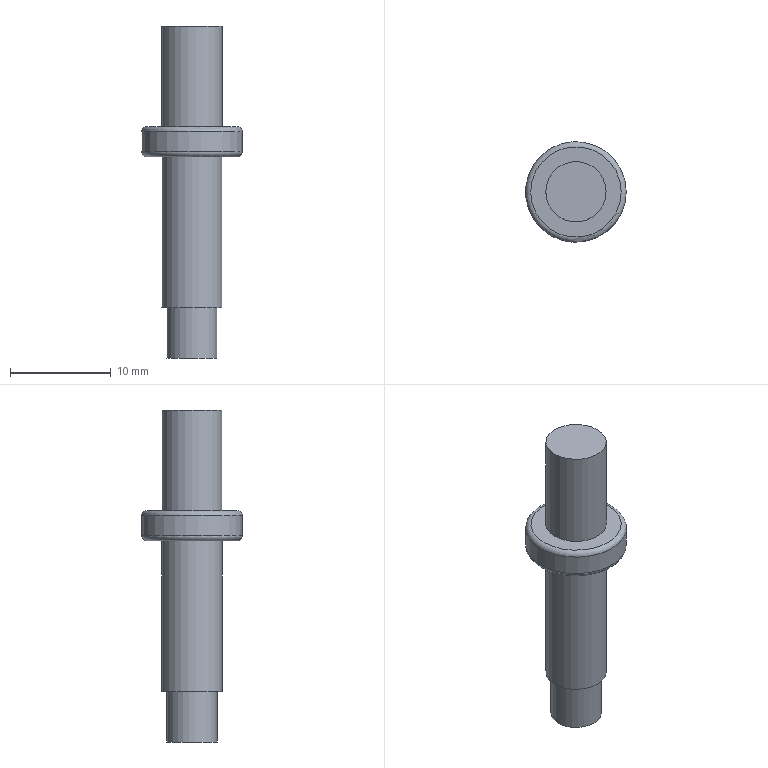Part | STEP file | 1-01.14 | 1 solid | 11 faces | box 10 x 10 x 33 mm | volume 1037 mm3 | plane 5 | cylinder 4 | torus 2 | commonest cylinder face diameters 6 x2 5 x1 10 x1
STEP:
#1=CARTESIAN_POINT('',(0.,0.,0.));
#2=DIRECTION('',(0.,0.,1.));
#3=DIRECTION('',(1.,0.,0.));
#4=AXIS2_PLACEMENT_3D('',#1,#2,#3);
#5=CARTESIAN_POINT('',(3.,0.,10.));
#6=VERTEX_POINT('',#5);
#7=CARTESIAN_POINT('',(0.,0.,10.));
#8=DIRECTION('',(0.,0.,1.));
#9=DIRECTION('',(1.,0.,0.));
#10=AXIS2_PLACEMENT_3D('',#7,#8,#9);
#11=CIRCLE('',#10,3.);
#12=CARTESIAN_POINT('',(-0.8038,0.,10.));
#13=DIRECTION('',(0.,0.,1.));
#14=DIRECTION('',(1.,0.,0.));
#15=AXIS2_PLACEMENT_3D('',#12,#13,#14);
#16=PLANE('',#15);
#17=CARTESIAN_POINT('',(0.8038,0.));
#18=DIRECTION('',(1.,0.));
#19=AXIS2_PLACEMENT_2D('',#17,#18);
#20=CIRCLE('',#19,3.);
#21=(GEOMETRIC_REPRESENTATION_CONTEXT(2)PARAMETRIC_REPRESENTATION_CONTEXT()REPRESENTATION_CONTEXT('',''));
#22=DEFINITIONAL_REPRESENTATION('',(#20),#21);
#23=PCURVE('',#16,#22);
#24=CARTESIAN_POINT('',(0.,0.,0.));
#25=DIRECTION('',(0.,0.,1.));
#26=DIRECTION('',(1.,0.,0.));
#27=AXIS2_PLACEMENT_3D('',#24,#25,#26);
#28=CYLINDRICAL_SURFACE('',#27,3.);
#29=CARTESIAN_POINT('',(0.,10.));
#30=DIRECTION('',(1.,0.));
#31=VECTOR('',#30,1.);
#32=LINE('',#29,#31);
#33=(GEOMETRIC_REPRESENTATION_CONTEXT(2)PARAMETRIC_REPRESENTATION_CONTEXT()REPRESENTATION_CONTEXT('',''));
#34=DEFINITIONAL_REPRESENTATION('',(#32),#33);
#35=PCURVE('',#28,#34);
#36=SURFACE_CURVE('',#11,(#23,#35),.PCURVE_S1.);
#37=EDGE_CURVE('',#6,#6,#36,.T.);
#38=ORIENTED_EDGE('',*,*,#37,.T.);
#39=EDGE_LOOP('',(#38));
#40=FACE_BOUND('',#39,.T.);
#41=ADVANCED_FACE('',(#40),#16,.T.);
#42=CARTESIAN_POINT('',(3.,0.,0.));
#43=VERTEX_POINT('',#42);
#44=CARTESIAN_POINT('',(0.,0.,0.));
#45=DIRECTION('',(0.,0.,1.));
#46=DIRECTION('',(1.,0.,0.));
#47=AXIS2_PLACEMENT_3D('',#44,#45,#46);
#48=CIRCLE('',#47,3.);
#49=CARTESIAN_POINT('',(0.,0.));
#50=DIRECTION('',(1.,0.));
#51=VECTOR('',#50,1.);
#52=LINE('',#49,#51);
#53=(GEOMETRIC_REPRESENTATION_CONTEXT(2)PARAMETRIC_REPRESENTATION_CONTEXT()REPRESENTATION_CONTEXT('',''));
#54=DEFINITIONAL_REPRESENTATION('',(#52),#53);
#55=PCURVE('',#28,#54);
#56=CARTESIAN_POINT('',(-1.34,0.,0.));
#57=DIRECTION('',(0.,0.,1.));
#58=DIRECTION('',(1.,0.,0.));
#59=AXIS2_PLACEMENT_3D('',#56,#57,#58);
#60=PLANE('',#59);
#61=CARTESIAN_POINT('',(1.34,0.));
#62=DIRECTION('',(1.,0.));
#63=AXIS2_PLACEMENT_2D('',#61,#62);
#64=CIRCLE('',#63,3.);
#65=(GEOMETRIC_REPRESENTATION_CONTEXT(2)PARAMETRIC_REPRESENTATION_CONTEXT()REPRESENTATION_CONTEXT('',''));
#66=DEFINITIONAL_REPRESENTATION('',(#64),#65);
#67=PCURVE('',#60,#66);
#68=SURFACE_CURVE('',#48,(#55,#67),.PCURVE_S1.);
#69=EDGE_CURVE('',#43,#43,#68,.T.);
#70=ORIENTED_EDGE('',*,*,#69,.T.);
#71=CARTESIAN_POINT('',(3.,0.,0.));
#72=DIRECTION('',(0.,0.,1.));
#73=VECTOR('',#72,1.);
#74=LINE('',#71,#73);
#75=CARTESIAN_POINT('',(6.283,0.));
#76=DIRECTION('',(0.,1.));
#77=VECTOR('',#76,1.);
#78=LINE('',#75,#77);
#79=(GEOMETRIC_REPRESENTATION_CONTEXT(2)PARAMETRIC_REPRESENTATION_CONTEXT()REPRESENTATION_CONTEXT('',''));
#80=DEFINITIONAL_REPRESENTATION('',(#78),#79);
#81=PCURVE('',#28,#80);
#82=CARTESIAN_POINT('',(0.,0.));
#83=DIRECTION('',(0.,1.));
#84=VECTOR('',#83,1.);
#85=LINE('',#82,#84);
#86=(GEOMETRIC_REPRESENTATION_CONTEXT(2)PARAMETRIC_REPRESENTATION_CONTEXT()REPRESENTATION_CONTEXT('',''));
#87=DEFINITIONAL_REPRESENTATION('',(#85),#86);
#88=PCURVE('',#28,#87);
#89=SEAM_CURVE('',#74,(#81,#88),.PCURVE_S1.);
#90=EDGE_CURVE('',#43,#6,#89,.T.);
#91=ORIENTED_EDGE('',*,*,#90,.T.);
#92=ORIENTED_EDGE('',*,*,#37,.F.);
#93=ORIENTED_EDGE('',*,*,#90,.F.);
#94=EDGE_LOOP('',(#70,#91,#92,#93));
#95=FACE_BOUND('',#94,.T.);
#96=ADVANCED_FACE('',(#95),#28,.T.);
#97=CARTESIAN_POINT('',(0.,-3.,-3.));
#98=VERTEX_POINT('',#97);
#99=CARTESIAN_POINT('',(0.,0.,-3.));
#100=DIRECTION('',(0.,0.,-1.));
#101=DIRECTION('',(0.,-1.,0.));
#102=AXIS2_PLACEMENT_3D('',#99,#100,#101);
#103=CIRCLE('',#102,3.);
#104=CARTESIAN_POINT('',(0.,0.,-3.));
#105=DIRECTION('',(0.,0.,-1.));
#106=DIRECTION('',(0.,-1.,0.));
#107=AXIS2_PLACEMENT_3D('',#104,#105,#106);
#108=CYLINDRICAL_SURFACE('',#107,3.);
#109=CARTESIAN_POINT('',(0.,0.));
#110=DIRECTION('',(1.,0.));
#111=VECTOR('',#110,1.);
#112=LINE('',#109,#111);
#113=(GEOMETRIC_REPRESENTATION_CONTEXT(2)PARAMETRIC_REPRESENTATION_CONTEXT()REPRESENTATION_CONTEXT('',''));
#114=DEFINITIONAL_REPRESENTATION('',(#112),#113);
#115=PCURVE('',#108,#114);
#116=CARTESIAN_POINT('',(-1.34,0.,-3.));
#117=DIRECTION('',(0.,0.,1.));
#118=DIRECTION('',(1.,0.,0.));
#119=AXIS2_PLACEMENT_3D('',#116,#117,#118);
#120=PLANE('',#119);
#121=CARTESIAN_POINT('',(1.34,-3.));
#122=CARTESIAN_POINT('',(-3.856,-3.));
#123=CARTESIAN_POINT('',(-1.258,1.5));
#124=CARTESIAN_POINT('',(1.34,6.));
#125=CARTESIAN_POINT('',(3.938,1.5));
#126=CARTESIAN_POINT('',(6.536,-3.));
#127=CARTESIAN_POINT('',(1.34,-3.));
#128=(BOUNDED_CURVE()B_SPLINE_CURVE(2,(#121,#122,#123,#124,#125,#126,#127),.UNSPECIFIED.,.T.,.F.)B_SPLINE_CURVE_WITH_KNOTS((1,2,2,2,2,1),(-2.094,0.,2.094,4.189,6.283,8.378),.UNSPECIFIED.)CURVE()GEOMETRIC_REPRESENTATION_ITEM()RATIONAL_B_SPLINE_CURVE((1.,0.5,1.,0.5,1.,0.5,1.))REPRESENTATION_ITEM(''));
#129=(GEOMETRIC_REPRESENTATION_CONTEXT(2)PARAMETRIC_REPRESENTATION_CONTEXT()REPRESENTATION_CONTEXT('',''));
#130=DEFINITIONAL_REPRESENTATION('',(#128),#129);
#131=PCURVE('',#120,#130);
#132=SURFACE_CURVE('',#103,(#115,#131),.PCURVE_S1.);
#133=EDGE_CURVE('',#98,#98,#132,.T.);
#134=ORIENTED_EDGE('',*,*,#133,.T.);
#135=CARTESIAN_POINT('',(0.,-3.,-18.));
#136=VERTEX_POINT('',#135);
#137=CARTESIAN_POINT('',(0.,-3.,-3.));
#138=DIRECTION('',(0.,0.,-1.));
#139=VECTOR('',#138,1.);
#140=LINE('',#137,#139);
#141=CARTESIAN_POINT('',(6.283,0.));
#142=DIRECTION('',(0.,1.));
#143=VECTOR('',#142,1.);
#144=LINE('',#141,#143);
#145=(GEOMETRIC_REPRESENTATION_CONTEXT(2)PARAMETRIC_REPRESENTATION_CONTEXT()REPRESENTATION_CONTEXT('',''));
#146=DEFINITIONAL_REPRESENTATION('',(#144),#145);
#147=PCURVE('',#108,#146);
#148=CARTESIAN_POINT('',(0.,0.));
#149=DIRECTION('',(0.,1.));
#150=VECTOR('',#149,1.);
#151=LINE('',#148,#150);
#152=(GEOMETRIC_REPRESENTATION_CONTEXT(2)PARAMETRIC_REPRESENTATION_CONTEXT()REPRESENTATION_CONTEXT('',''));
#153=DEFINITIONAL_REPRESENTATION('',(#151),#152);
#154=PCURVE('',#108,#153);
#155=SEAM_CURVE('',#140,(#147,#154),.PCURVE_S1.);
#156=EDGE_CURVE('',#98,#136,#155,.T.);
#157=ORIENTED_EDGE('',*,*,#156,.T.);
#158=CARTESIAN_POINT('',(0.,0.,-18.));
#159=DIRECTION('',(0.,0.,-1.));
#160=DIRECTION('',(0.,-1.,0.));
#161=AXIS2_PLACEMENT_3D('',#158,#159,#160);
#162=CIRCLE('',#161,3.);
#163=CARTESIAN_POINT('',(0.,15.));
#164=DIRECTION('',(1.,0.));
#165=VECTOR('',#164,1.);
#166=LINE('',#163,#165);
#167=(GEOMETRIC_REPRESENTATION_CONTEXT(2)PARAMETRIC_REPRESENTATION_CONTEXT()REPRESENTATION_CONTEXT('',''));
#168=DEFINITIONAL_REPRESENTATION('',(#166),#167);
#169=PCURVE('',#108,#168);
#170=CARTESIAN_POINT('',(0.,0.8038,-18.));
#171=DIRECTION('',(0.,0.,-1.));
#172=DIRECTION('',(0.,-1.,0.));
#173=AXIS2_PLACEMENT_3D('',#170,#171,#172);
#174=PLANE('',#173);
#175=CARTESIAN_POINT('',(0.8038,0.));
#176=DIRECTION('',(1.,0.));
#177=AXIS2_PLACEMENT_2D('',#175,#176);
#178=CIRCLE('',#177,3.);
#179=(GEOMETRIC_REPRESENTATION_CONTEXT(2)PARAMETRIC_REPRESENTATION_CONTEXT()REPRESENTATION_CONTEXT('',''));
#180=DEFINITIONAL_REPRESENTATION('',(#178),#179);
#181=PCURVE('',#174,#180);
#182=SURFACE_CURVE('',#162,(#169,#181),.PCURVE_S1.);
#183=EDGE_CURVE('',#136,#136,#182,.T.);
#184=ORIENTED_EDGE('',*,*,#183,.F.);
#185=ORIENTED_EDGE('',*,*,#156,.F.);
#186=EDGE_LOOP('',(#134,#157,#184,#185));
#187=FACE_BOUND('',#186,.T.);
#188=ADVANCED_FACE('',(#187),#108,.T.);
#189=ORIENTED_EDGE('',*,*,#183,.T.);
#190=EDGE_LOOP('',(#189));
#191=FACE_BOUND('',#190,.T.);
#192=CARTESIAN_POINT('',(0.,-2.5,-18.));
#193=VERTEX_POINT('',#192);
#194=CARTESIAN_POINT('',(0.,0.,-18.));
#195=DIRECTION('',(0.,0.,-1.));
#196=DIRECTION('',(0.,-1.,0.));
#197=AXIS2_PLACEMENT_3D('',#194,#195,#196);
#198=CIRCLE('',#197,2.5);
#199=CARTESIAN_POINT('',(0.8038,0.));
#200=DIRECTION('',(1.,0.));
#201=AXIS2_PLACEMENT_2D('',#199,#200);
#202=CIRCLE('',#201,2.5);
#203=(GEOMETRIC_REPRESENTATION_CONTEXT(2)PARAMETRIC_REPRESENTATION_CONTEXT()REPRESENTATION_CONTEXT('',''));
#204=DEFINITIONAL_REPRESENTATION('',(#202),#203);
#205=PCURVE('',#174,#204);
#206=CARTESIAN_POINT('',(0.,0.,-18.));
#207=DIRECTION('',(0.,0.,-1.));
#208=DIRECTION('',(0.,-1.,0.));
#209=AXIS2_PLACEMENT_3D('',#206,#207,#208);
#210=CYLINDRICAL_SURFACE('',#209,2.5);
#211=CARTESIAN_POINT('',(0.,0.));
#212=DIRECTION('',(1.,0.));
#213=VECTOR('',#212,1.);
#214=LINE('',#211,#213);
#215=(GEOMETRIC_REPRESENTATION_CONTEXT(2)PARAMETRIC_REPRESENTATION_CONTEXT()REPRESENTATION_CONTEXT('',''));
#216=DEFINITIONAL_REPRESENTATION('',(#214),#215);
#217=PCURVE('',#210,#216);
#218=SURFACE_CURVE('',#198,(#205,#217),.PCURVE_S1.);
#219=EDGE_CURVE('',#193,#193,#218,.T.);
#220=ORIENTED_EDGE('',*,*,#219,.F.);
#221=EDGE_LOOP('',(#220));
#222=FACE_BOUND('',#221,.T.);
#223=ADVANCED_FACE('',(#191,#222),#174,.T.);
#224=ORIENTED_EDGE('',*,*,#219,.T.);
#225=CARTESIAN_POINT('',(0.,-2.5,-23.));
#226=VERTEX_POINT('',#225);
#227=CARTESIAN_POINT('',(0.,-2.5,-18.));
#228=DIRECTION('',(0.,0.,-1.));
#229=VECTOR('',#228,1.);
#230=LINE('',#227,#229);
#231=CARTESIAN_POINT('',(6.283,0.));
#232=DIRECTION('',(0.,1.));
#233=VECTOR('',#232,1.);
#234=LINE('',#231,#233);
#235=(GEOMETRIC_REPRESENTATION_CONTEXT(2)PARAMETRIC_REPRESENTATION_CONTEXT()REPRESENTATION_CONTEXT('',''));
#236=DEFINITIONAL_REPRESENTATION('',(#234),#235);
#237=PCURVE('',#210,#236);
#238=CARTESIAN_POINT('',(0.,0.));
#239=DIRECTION('',(0.,1.));
#240=VECTOR('',#239,1.);
#241=LINE('',#238,#240);
#242=(GEOMETRIC_REPRESENTATION_CONTEXT(2)PARAMETRIC_REPRESENTATION_CONTEXT()REPRESENTATION_CONTEXT('',''));
#243=DEFINITIONAL_REPRESENTATION('',(#241),#242);
#244=PCURVE('',#210,#243);
#245=SEAM_CURVE('',#230,(#237,#244),.PCURVE_S1.);
#246=EDGE_CURVE('',#193,#226,#245,.T.);
#247=ORIENTED_EDGE('',*,*,#246,.T.);
#248=CARTESIAN_POINT('',(0.,0.,-23.));
#249=DIRECTION('',(0.,0.,-1.));
#250=DIRECTION('',(0.,-1.,0.));
#251=AXIS2_PLACEMENT_3D('',#248,#249,#250);
#252=CIRCLE('',#251,2.5);
#253=CARTESIAN_POINT('',(0.,5.));
#254=DIRECTION('',(1.,0.));
#255=VECTOR('',#254,1.);
#256=LINE('',#253,#255);
#257=(GEOMETRIC_REPRESENTATION_CONTEXT(2)PARAMETRIC_REPRESENTATION_CONTEXT()REPRESENTATION_CONTEXT('',''));
#258=DEFINITIONAL_REPRESENTATION('',(#256),#257);
#259=PCURVE('',#210,#258);
#260=CARTESIAN_POINT('',(0.,0.6699,-23.));
#261=DIRECTION('',(0.,0.,-1.));
#262=DIRECTION('',(0.,-1.,0.));
#263=AXIS2_PLACEMENT_3D('',#260,#261,#262);
#264=PLANE('',#263);
#265=CARTESIAN_POINT('',(0.6699,0.));
#266=DIRECTION('',(1.,0.));
#267=AXIS2_PLACEMENT_2D('',#265,#266);
#268=CIRCLE('',#267,2.5);
#269=(GEOMETRIC_REPRESENTATION_CONTEXT(2)PARAMETRIC_REPRESENTATION_CONTEXT()REPRESENTATION_CONTEXT('',''));
#270=DEFINITIONAL_REPRESENTATION('',(#268),#269);
#271=PCURVE('',#264,#270);
#272=SURFACE_CURVE('',#252,(#259,#271),.PCURVE_S1.);
#273=EDGE_CURVE('',#226,#226,#272,.T.);
#274=ORIENTED_EDGE('',*,*,#273,.F.);
#275=ORIENTED_EDGE('',*,*,#246,.F.);
#276=EDGE_LOOP('',(#224,#247,#274,#275));
#277=FACE_BOUND('',#276,.T.);
#278=ADVANCED_FACE('',(#277),#210,.T.);
#279=ORIENTED_EDGE('',*,*,#273,.T.);
#280=EDGE_LOOP('',(#279));
#281=FACE_BOUND('',#280,.T.);
#282=ADVANCED_FACE('',(#281),#264,.T.);
#283=CARTESIAN_POINT('',(4.5,0.,0.));
#284=VERTEX_POINT('',#283);
#285=CARTESIAN_POINT('',(0.,0.,0.));
#286=DIRECTION('',(0.,0.,1.));
#287=DIRECTION('',(1.,0.,0.));
#288=AXIS2_PLACEMENT_3D('',#285,#286,#287);
#289=CIRCLE('',#288,4.5);
#290=CARTESIAN_POINT('',(1.34,0.));
#291=DIRECTION('',(1.,0.));
#292=AXIS2_PLACEMENT_2D('',#290,#291);
#293=CIRCLE('',#292,4.5);
#294=(GEOMETRIC_REPRESENTATION_CONTEXT(2)PARAMETRIC_REPRESENTATION_CONTEXT()REPRESENTATION_CONTEXT('',''));
#295=DEFINITIONAL_REPRESENTATION('',(#293),#294);
#296=PCURVE('',#60,#295);
#297=CARTESIAN_POINT('',(0.,0.,-0.5));
#298=DIRECTION('',(0.,0.,-1.));
#299=DIRECTION('',(1.,0.,0.));
#300=AXIS2_PLACEMENT_3D('',#297,#298,#299);
#301=TOROIDAL_SURFACE('',#300,4.5,0.5);
#302=CARTESIAN_POINT('',(6.283,4.712));
#303=DIRECTION('',(-1.,0.));
#304=VECTOR('',#303,1.);
#305=LINE('',#302,#304);
#306=(GEOMETRIC_REPRESENTATION_CONTEXT(2)PARAMETRIC_REPRESENTATION_CONTEXT()REPRESENTATION_CONTEXT('',''));
#307=DEFINITIONAL_REPRESENTATION('',(#305),#306);
#308=PCURVE('',#301,#307);
#309=SURFACE_CURVE('',#289,(#296,#308),.PCURVE_S1.);
#310=EDGE_CURVE('',#284,#284,#309,.T.);
#311=ORIENTED_EDGE('',*,*,#310,.T.);
#312=EDGE_LOOP('',(#311));
#313=FACE_BOUND('',#312,.T.);
#314=ORIENTED_EDGE('',*,*,#69,.F.);
#315=EDGE_LOOP('',(#314));
#316=FACE_BOUND('',#315,.T.);
#317=ADVANCED_FACE('',(#313,#316),#60,.T.);
#318=CARTESIAN_POINT('',(5.,0.,-0.5));
#319=VERTEX_POINT('',#318);
#320=CARTESIAN_POINT('',(0.,0.,-0.5));
#321=DIRECTION('',(0.,0.,1.));
#322=DIRECTION('',(1.,0.,0.));
#323=AXIS2_PLACEMENT_3D('',#320,#321,#322);
#324=CIRCLE('',#323,5.);
#325=CARTESIAN_POINT('',(0.,0.,0.));
#326=DIRECTION('',(0.,0.,-1.));
#327=DIRECTION('',(1.,0.,0.));
#328=AXIS2_PLACEMENT_3D('',#325,#326,#327);
#329=CYLINDRICAL_SURFACE('',#328,5.);
#330=CARTESIAN_POINT('',(6.283,0.5));
#331=DIRECTION('',(-1.,0.));
#332=VECTOR('',#331,1.);
#333=LINE('',#330,#332);
#334=(GEOMETRIC_REPRESENTATION_CONTEXT(2)PARAMETRIC_REPRESENTATION_CONTEXT()REPRESENTATION_CONTEXT('',''));
#335=DEFINITIONAL_REPRESENTATION('',(#333),#334);
#336=PCURVE('',#329,#335);
#337=CARTESIAN_POINT('',(6.283,6.283));
#338=DIRECTION('',(-1.,0.));
#339=VECTOR('',#338,1.);
#340=LINE('',#337,#339);
#341=(GEOMETRIC_REPRESENTATION_CONTEXT(2)PARAMETRIC_REPRESENTATION_CONTEXT()REPRESENTATION_CONTEXT('',''));
#342=DEFINITIONAL_REPRESENTATION('',(#340),#341);
#343=PCURVE('',#301,#342);
#344=SURFACE_CURVE('',#324,(#336,#343),.PCURVE_S1.);
#345=EDGE_CURVE('',#319,#319,#344,.T.);
#346=ORIENTED_EDGE('',*,*,#345,.F.);
#347=CARTESIAN_POINT('',(5.,0.,-2.5));
#348=VERTEX_POINT('',#347);
#349=CARTESIAN_POINT('',(5.,0.,-0.5));
#350=DIRECTION('',(0.,0.,-1.));
#351=VECTOR('',#350,1.);
#352=LINE('',#349,#351);
#353=CARTESIAN_POINT('',(6.283,0.5));
#354=DIRECTION('',(0.,1.));
#355=VECTOR('',#354,1.);
#356=LINE('',#353,#355);
#357=(GEOMETRIC_REPRESENTATION_CONTEXT(2)PARAMETRIC_REPRESENTATION_CONTEXT()REPRESENTATION_CONTEXT('',''));
#358=DEFINITIONAL_REPRESENTATION('',(#356),#357);
#359=PCURVE('',#329,#358);
#360=CARTESIAN_POINT('',(0.,0.5));
#361=DIRECTION('',(0.,1.));
#362=VECTOR('',#361,1.);
#363=LINE('',#360,#362);
#364=(GEOMETRIC_REPRESENTATION_CONTEXT(2)PARAMETRIC_REPRESENTATION_CONTEXT()REPRESENTATION_CONTEXT('',''));
#365=DEFINITIONAL_REPRESENTATION('',(#363),#364);
#366=PCURVE('',#329,#365);
#367=SEAM_CURVE('',#352,(#359,#366),.PCURVE_S1.);
#368=EDGE_CURVE('',#319,#348,#367,.T.);
#369=ORIENTED_EDGE('',*,*,#368,.T.);
#370=CARTESIAN_POINT('',(0.,0.,-2.5));
#371=DIRECTION('',(0.,0.,1.));
#372=DIRECTION('',(1.,0.,0.));
#373=AXIS2_PLACEMENT_3D('',#370,#371,#372);
#374=CIRCLE('',#373,5.);
#375=CARTESIAN_POINT('',(6.283,2.5));
#376=DIRECTION('',(-1.,0.));
#377=VECTOR('',#376,1.);
#378=LINE('',#375,#377);
#379=(GEOMETRIC_REPRESENTATION_CONTEXT(2)PARAMETRIC_REPRESENTATION_CONTEXT()REPRESENTATION_CONTEXT('',''));
#380=DEFINITIONAL_REPRESENTATION('',(#378),#379);
#381=PCURVE('',#329,#380);
#382=CARTESIAN_POINT('',(0.,0.,-2.5));
#383=DIRECTION('',(0.,0.,-1.));
#384=DIRECTION('',(1.,0.,0.));
#385=AXIS2_PLACEMENT_3D('',#382,#383,#384);
#386=TOROIDAL_SURFACE('',#385,4.5,0.5);
#387=CARTESIAN_POINT('',(6.283,0.));
#388=DIRECTION('',(-1.,0.));
#389=VECTOR('',#388,1.);
#390=LINE('',#387,#389);
#391=(GEOMETRIC_REPRESENTATION_CONTEXT(2)PARAMETRIC_REPRESENTATION_CONTEXT()REPRESENTATION_CONTEXT('',''));
#392=DEFINITIONAL_REPRESENTATION('',(#390),#391);
#393=PCURVE('',#386,#392);
#394=SURFACE_CURVE('',#374,(#381,#393),.PCURVE_S1.);
#395=EDGE_CURVE('',#348,#348,#394,.T.);
#396=ORIENTED_EDGE('',*,*,#395,.T.);
#397=ORIENTED_EDGE('',*,*,#368,.F.);
#398=EDGE_LOOP('',(#346,#369,#396,#397));
#399=FACE_BOUND('',#398,.T.);
#400=ADVANCED_FACE('',(#399),#329,.T.);
#401=CARTESIAN_POINT('',(4.5,0.,-3.));
#402=VERTEX_POINT('',#401);
#403=CARTESIAN_POINT('',(0.,0.,-3.));
#404=DIRECTION('',(0.,0.,1.));
#405=DIRECTION('',(1.,0.,0.));
#406=AXIS2_PLACEMENT_3D('',#403,#404,#405);
#407=CIRCLE('',#406,4.5);
#408=CARTESIAN_POINT('',(1.34,0.));
#409=DIRECTION('',(1.,0.));
#410=AXIS2_PLACEMENT_2D('',#408,#409);
#411=CIRCLE('',#410,4.5);
#412=(GEOMETRIC_REPRESENTATION_CONTEXT(2)PARAMETRIC_REPRESENTATION_CONTEXT()REPRESENTATION_CONTEXT('',''));
#413=DEFINITIONAL_REPRESENTATION('',(#411),#412);
#414=PCURVE('',#120,#413);
#415=CARTESIAN_POINT('',(6.283,1.571));
#416=DIRECTION('',(-1.,0.));
#417=VECTOR('',#416,1.);
#418=LINE('',#415,#417);
#419=(GEOMETRIC_REPRESENTATION_CONTEXT(2)PARAMETRIC_REPRESENTATION_CONTEXT()REPRESENTATION_CONTEXT('',''));
#420=DEFINITIONAL_REPRESENTATION('',(#418),#419);
#421=PCURVE('',#386,#420);
#422=SURFACE_CURVE('',#407,(#414,#421),.PCURVE_S1.);
#423=EDGE_CURVE('',#402,#402,#422,.T.);
#424=ORIENTED_EDGE('',*,*,#423,.T.);
#425=EDGE_LOOP('',(#424));
#426=FACE_BOUND('',#425,.F.);
#427=ORIENTED_EDGE('',*,*,#133,.T.);
#428=EDGE_LOOP('',(#427));
#429=FACE_BOUND('',#428,.F.);
#430=ADVANCED_FACE('',(#426,#429),#120,.F.);
#431=ORIENTED_EDGE('',*,*,#310,.F.);
#432=CARTESIAN_POINT('',(4.5,0.,-0.5));
#433=DIRECTION('',(0.,1.,0.));
#434=DIRECTION('',(0.,0.,1.));
#435=AXIS2_PLACEMENT_3D('',#432,#433,#434);
#436=CIRCLE('',#435,0.5);
#437=CARTESIAN_POINT('',(6.283,4.712));
#438=DIRECTION('',(0.,1.));
#439=VECTOR('',#438,1.);
#440=LINE('',#437,#439);
#441=(GEOMETRIC_REPRESENTATION_CONTEXT(2)PARAMETRIC_REPRESENTATION_CONTEXT()REPRESENTATION_CONTEXT('',''));
#442=DEFINITIONAL_REPRESENTATION('',(#440),#441);
#443=PCURVE('',#301,#442);
#444=CARTESIAN_POINT('',(0.,4.712));
#445=DIRECTION('',(0.,1.));
#446=VECTOR('',#445,1.);
#447=LINE('',#444,#446);
#448=(GEOMETRIC_REPRESENTATION_CONTEXT(2)PARAMETRIC_REPRESENTATION_CONTEXT()REPRESENTATION_CONTEXT('',''));
#449=DEFINITIONAL_REPRESENTATION('',(#447),#448);
#450=PCURVE('',#301,#449);
#451=SEAM_CURVE('',#436,(#443,#450),.PCURVE_S1.);
#452=EDGE_CURVE('',#284,#319,#451,.T.);
#453=ORIENTED_EDGE('',*,*,#452,.T.);
#454=ORIENTED_EDGE('',*,*,#345,.T.);
#455=ORIENTED_EDGE('',*,*,#452,.F.);
#456=EDGE_LOOP('',(#431,#453,#454,#455));
#457=FACE_BOUND('',#456,.T.);
#458=ADVANCED_FACE('',(#457),#301,.T.);
#459=CARTESIAN_POINT('',(4.5,0.,-2.5));
#460=DIRECTION('',(0.,-1.,0.));
#461=DIRECTION('',(0.,0.,-1.));
#462=AXIS2_PLACEMENT_3D('',#459,#460,#461);
#463=CIRCLE('',#462,0.5);
#464=CARTESIAN_POINT('',(0.,1.571));
#465=DIRECTION('',(0.,-1.));
#466=VECTOR('',#465,1.);
#467=LINE('',#464,#466);
#468=(GEOMETRIC_REPRESENTATION_CONTEXT(2)PARAMETRIC_REPRESENTATION_CONTEXT()REPRESENTATION_CONTEXT('',''));
#469=DEFINITIONAL_REPRESENTATION('',(#467),#468);
#470=PCURVE('',#386,#469);
#471=CARTESIAN_POINT('',(6.283,1.571));
#472=DIRECTION('',(0.,-1.));
#473=VECTOR('',#472,1.);
#474=LINE('',#471,#473);
#475=(GEOMETRIC_REPRESENTATION_CONTEXT(2)PARAMETRIC_REPRESENTATION_CONTEXT()REPRESENTATION_CONTEXT('',''));
#476=DEFINITIONAL_REPRESENTATION('',(#474),#475);
#477=PCURVE('',#386,#476);
#478=SEAM_CURVE('',#463,(#470,#477),.PCURVE_S1.);
#479=EDGE_CURVE('',#402,#348,#478,.T.);
#480=ORIENTED_EDGE('',*,*,#479,.T.);
#481=ORIENTED_EDGE('',*,*,#395,.F.);
#482=ORIENTED_EDGE('',*,*,#479,.F.);
#483=ORIENTED_EDGE('',*,*,#423,.T.);
#484=EDGE_LOOP('',(#480,#481,#482,#483));
#485=FACE_BOUND('',#484,.T.);
#486=ADVANCED_FACE('',(#485),#386,.T.);
#487=CLOSED_SHELL('',(#41,#96,#188,#223,#278,#282,#317,#400,#430,#458,#486));
#488=MANIFOLD_SOLID_BREP('',#487);
#489=(LENGTH_UNIT()NAMED_UNIT(*)SI_UNIT(.MILLI.,.METRE.));
#490=UNCERTAINTY_MEASURE_WITH_UNIT(LENGTH_MEASURE(0.0000001),#489,'','');
#491=(NAMED_UNIT(*)PLANE_ANGLE_UNIT()SI_UNIT($,.RADIAN.));
#492=(NAMED_UNIT(*)SI_UNIT($,.STERADIAN.)SOLID_ANGLE_UNIT());
#493=(GEOMETRIC_REPRESENTATION_CONTEXT(3)GLOBAL_UNCERTAINTY_ASSIGNED_CONTEXT((#490))GLOBAL_UNIT_ASSIGNED_CONTEXT((#489,#491,#492))REPRESENTATION_CONTEXT('',''));
#494=ADVANCED_BREP_SHAPE_REPRESENTATION('',(#4,#488),#493);